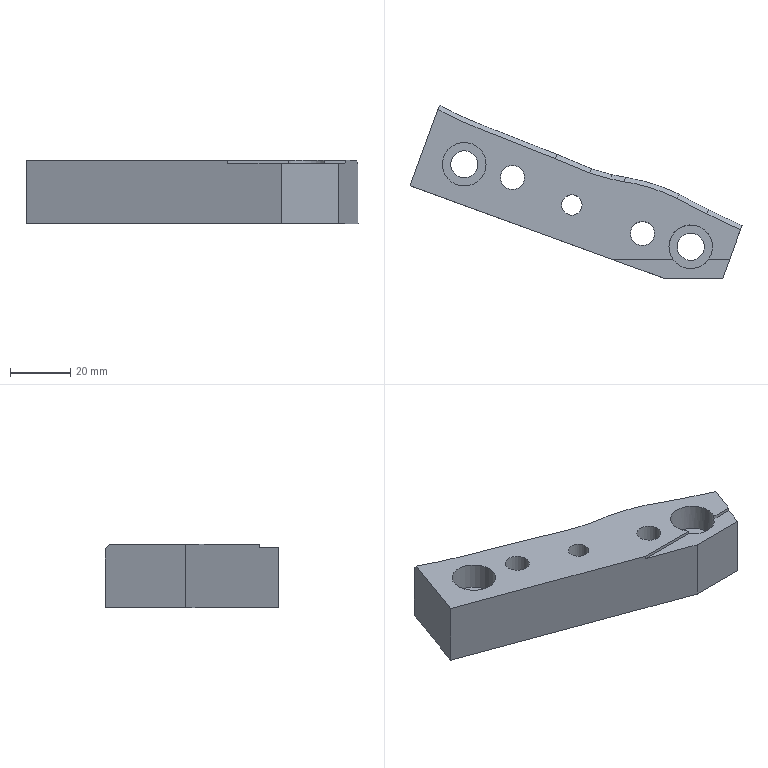Part | NX | features 23 2 | 1 solid | 33 faces | box 110.132 x 57.627 x 21 mm | volume 52214 mm3 | plane 16 | spline 10 | cylinder 7 | commonest cylinder face diameters 8.001 x2 9 x2 14.5 x2 6.8 x1